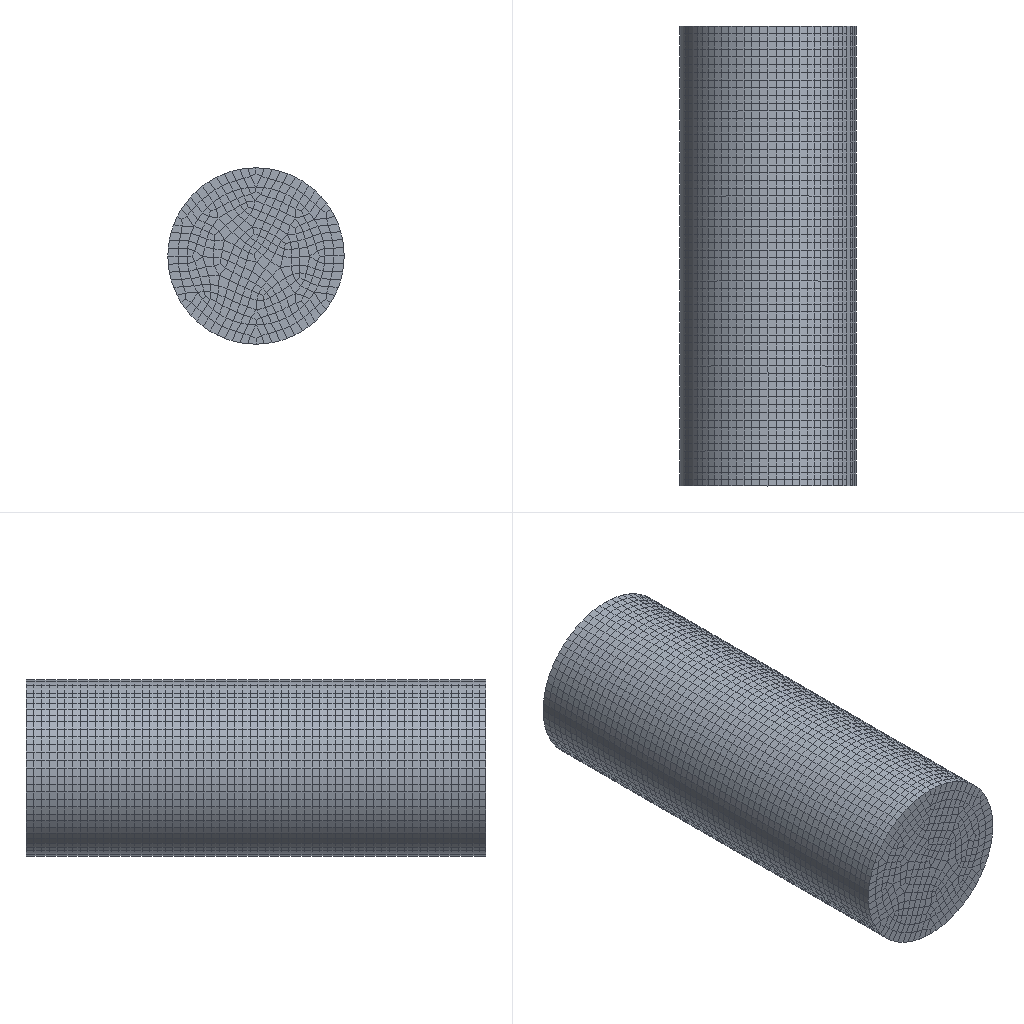Simulation study | ansys workbench
Ansys APDL input file, long lists of numbers shortened:
/batch
/config,noeldb,1     ! force off writing results to database
*get,_wallstrt,active,,time,wall
! ANSYS input file written by Workbench version 2020 R2
! File used for geometry attach:
/title,unsaved_project--___ (A5)
*DIM,_wb_ProjectScratch_dir,string,248
_wb_ProjectScratch_dir(1) = ''
*DIM,_wb_SolverFiles_dir,string,248
_wb_SolverFiles_dir(1) = ''
*DIM,_wb_userfiles_dir,string,248
_wb_userfiles_dir(1) = ''
/com,--- Data in consistent MKS units. See Solving Units in the help system for more information.
/units,MKS
/nopr
/wb,file,start              !  signify a WB generated input file
/prep7
! Turn off shape checking because checks already performed inside WB mesher.
! See help system for more information.
SHPP,OFF,,NOWARN
/nolist
etcon,set             ! allow ANSYS to choose best KEYOP's for 180x elements
/com,*********** Nodes for the whole assembly ***********
nblock,3,,50740
(1i9,3e20.9e3)
        1    -1.192148224E-02     0.000000000E+00    -1.104059469E-02
! (46127 more lines like these left out)
-1
/wb,elem,start            !  set before creation of elements
/com,*********** Elements for Body 1 "SYS\__" ***********
et,1,90
eblock,19,solid,,8511
(19i9)
        1        1        1        1        0        0        0        0       20        0        1      424      532    12288    12285      422      531    12424    12421
! (17021 more lines like these left out)
-1
/wb,elem,end               !  done creating elements
/com,*********** Send User Defined Coordinate System(s) ***********
csys,0
toffst,273.15,  ! Temperature offset from absolute zero
/wb,mat,start              !  starting to send materials
/com,*********** Send Materials ***********
Temperature = 'TEMP' ! Temperature
MP,DENS,1,7850,	! kg m^-3
MP,ALPX,1,1.2e-05,	! C^-1
MP,C,1,434,	! J kg^-1 C^-1
MP,KXX,1,60.5,	! W m^-1 C^-1
MP,RSVX,1,1.7e-07,	! kg m^3 A^-2 s^-3
MP,EX,1,200000000000,	! Pa
MP,NUXY,1,0.3,
MP,MURX,1,10000,
/wb,mat,end                !  done sending materials
!************************* Model Summary ********************
!SYS\__,	Structural Steel,	matid,	1
!************************* End Model Summary ********************
! get the diagonal of the bounding box. Needed later for other things
*get,_xmin,node,,mnloc,x
*get,_ymin,node,,mnloc,y
*get,_zmin,node,,mnloc,z
*get,_xmax,node,,mxloc,x
*get,_ymax,node,,mxloc,y
*get,_zmax,node,,mxloc,z
_ASMDIAG=(_xmax-_xmin)*(_xmax-_xmin)+(_ymax-_ymin)*(_ymax-_ymin)+(_zmax-_zmin)*(_zmax-_zmin)
_ASMDIAG=SQRT(_ASMDIAG)
/wb,contact,start          !  starting to send contact
/wb,contact,end            !  done creating contacts
/golist
/wb,load,start             !  starting to send loads
/com,*********** Define Temperature Constraint ***********
CMBLOCK,_CM33   ,NODE,    10344
(8i10)
       799       800       801       802       803       804       805       806
! (1292 more lines like these left out)
*DIM,_loadvari33,TABLE,2,1,1,TIME,
! Time values
_loadvari33(1,0,1) = 0.
_loadvari33(2,0,1) = 1.
! Load values
_loadvari33(1,1,1) = 100.
_loadvari33(2,1,1) = 100.
fcum,add                   ! add nodal forces up (needed in case have loads on the same edge,vertex)
fcum                       ! reset default on fcum command since done sending WB F loads
/com,*********** Create "______" ***********
et,2,152
eblock,10,,,4080
(15i9)
    16518        2        2        2        0    12215    12217    12081    12079    45179    45178    44727    45173
! (4079 more lines like these left out)
-1
esel,s,type,,2
keyop,2,8,2.
keyop,2,13,0
esel,all
/com,***************** Define Uniform Initial temperature ***************
tunif,22.
/gst,on,on
fini
*get,_numnode,node,0,count
*get,_numelem,elem,0,count
*get, _MAXELEMNUM, elem, 0, NUM, MAX
*get, _MAXNODENUM, node, 0, NUM, MAX
*get, _MAXELEMTYPE, etyp, 0, NUM, MAX
*get, _MAXREALCONST, real, 0, NUM, MAX
/go
/wb,load,end               !  done creating loads
/com,--- Number of total nodes = %_numnode%
/com,--- Number of contact elements = 4080
/com,--- Number of spring elements = 0
/com,--- Number of bearing elements = 0
/com,--- Number of solid elements = 8511
/com,--- Number of condensed parts = 0
/com,--- Number of total elements = %_numelem%
*get,_wallbsol,active,,time,wall
/com,****************************************************************************
/com,*************************    SOLUTION       ********************************
/com,****************************************************************************
/solu
antype,0                   ! static analysis
!eqsl,sparse               ! using sparse solver which is default so no eqsl command needed
cntr,print,1               ! print out contact info and also make no initial contact an error
rescontrol,,none                 ! Do not keep any restart files
/com,****************************************************
/com,******************* SOLVE FOR LS 1 OF 1 ****************
d,_CM33,temp,%_loadvari33%
esel,s,type,,2
nsle
sf,all,conv,250.,22.
nsel,all
esel,all
autots,on
nsub,1,10,1
time,1.
outres,erase
outres,all,none
outres,nsol,all
outres,rsol,all
outres,eangl,all
outres,veng,all
outres,fflux,all
outres,cont,all
/nopr
esel,s,type,,2
cm,_elmisc,elem
esel,all
/gopr
outres,misc,all,_elmisc
cnvtol,heat,,.001,,1.e-006    ! Program Controlled. Set MINREF equivalent of 1e-6 Watts
! *********** WB SOLVE COMMAND ***********
! check interactive state
*get,ANSINTER_,active,,int
*if,ANSINTER_,ne,0,then
/eof
*endif
solve
/com *************** Write FE CONNECTORS *********
CEWRITE,file,ce,,INTE
/com,****************************************************
/com,*************** FINISHED SOLVE FOR LS 1 *************
*get,_wallasol,active,,time,wall
/post1
xmlo,ENCODING,ISO-8859-1
xmlo,parm
/xml,parm,xml
fini
/gopr
*get,_walldone,active,,time,wall
_preptime=(_wallbsol-_wallstrt)*3600
_solvtime=(_wallasol-_wallbsol)*3600
_posttime=(_walldone-_wallasol)*3600
_totaltim=(_walldone-_wallstrt)*3600
*get,_dlbratio,active,0,solu,dlbr
*get,_combtime,active,0,solu,comb
/com,--- Total number of nodes = %_numnode%
/com,--- Total number of elements = %_numelem%
/com,--- Element load balance ratio = %_dlbratio%
/com,--- Time to combine distributed files = %_combtime%
/wb,file,end               ! done with WB generated input